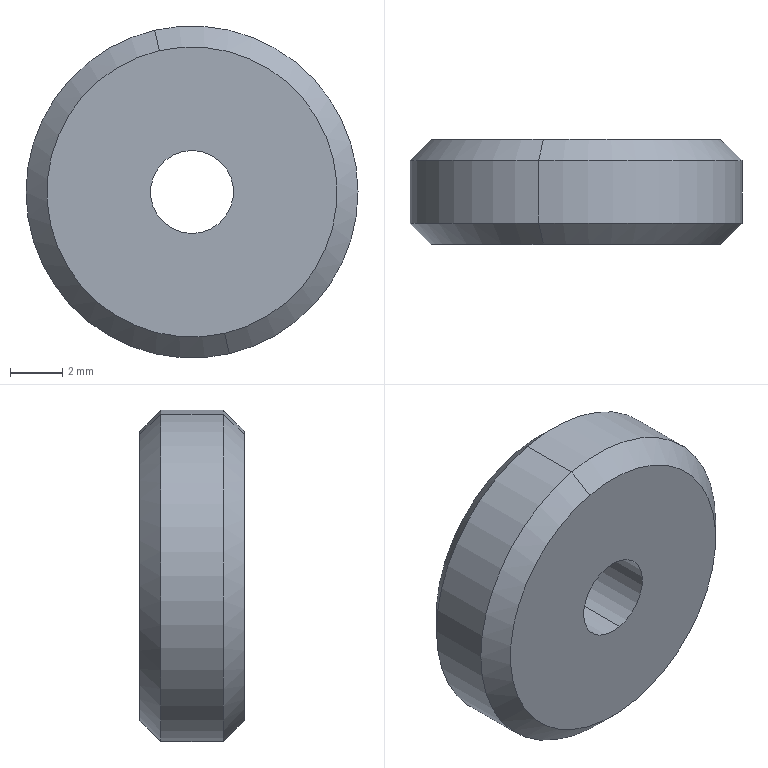Part | STEP file | 4-20.sldasm-Part-188 | 1 solid | 10 faces | box 12.7 x 4 x 12.7 mm | volume 450.576 mm3 | cone 4 | cylinder 4 | plane 2 | commonest cylinder face diameters 3.175 x2 12.7 x2
STEP:
#1=CARTESIAN_POINT('',(-144.626,-599.425,-33.06));
#2=VERTEX_POINT('',#1);
#3=CARTESIAN_POINT('',(-147.122,-599.425,-22.244));
#4=VERTEX_POINT('',#3);
#5=CARTESIAN_POINT('',(-145.874,-599.425,-27.652));
#6=DIRECTION('',(0.,-1.,0.));
#7=DIRECTION('',(-0.225,0.,0.9744));
#8=AXIS2_PLACEMENT_3D('',#5,#6,#7);
#9=CIRCLE('',#8,5.55);
#10=EDGE_CURVE('',#2,#4,#9,.T.);
#11=ORIENTED_EDGE('',*,*,#10,.F.);
#12=CARTESIAN_POINT('',(-144.446,-598.625,-33.84));
#13=VERTEX_POINT('',#12);
#14=CARTESIAN_POINT('',(-144.626,-599.425,-33.06));
#15=DIRECTION('',(0.1591,0.7071,-0.689));
#16=VECTOR('',#15,1000.);
#17=LINE('',#14,#16);
#18=EDGE_CURVE('',#2,#13,#17,.T.);
#19=ORIENTED_EDGE('',*,*,#18,.T.);
#20=CARTESIAN_POINT('',(-147.302,-598.625,-21.465));
#21=VERTEX_POINT('',#20);
#22=CARTESIAN_POINT('',(-145.874,-598.625,-27.652));
#23=DIRECTION('',(0.,1.,0.));
#24=DIRECTION('',(0.225,0.,-0.9744));
#25=AXIS2_PLACEMENT_3D('',#22,#23,#24);
#26=CIRCLE('',#25,6.35);
#27=EDGE_CURVE('',#21,#13,#26,.T.);
#28=ORIENTED_EDGE('',*,*,#27,.F.);
#29=CARTESIAN_POINT('',(-147.122,-599.425,-22.244));
#30=DIRECTION('',(-0.1591,0.7071,0.689));
#31=VECTOR('',#30,1000.);
#32=LINE('',#29,#31);
#33=EDGE_CURVE('',#4,#21,#32,.T.);
#34=ORIENTED_EDGE('',*,*,#33,.F.);
#35=EDGE_LOOP('',(#11,#19,#28,#34));
#36=FACE_OUTER_BOUND('',#35,.T.);
#37=CARTESIAN_POINT('',(-145.874,-599.425,-27.652));
#38=DIRECTION('',(0.,1.,0.));
#39=DIRECTION('',(-0.225,0.,0.9744));
#40=AXIS2_PLACEMENT_3D('',#37,#38,#39);
#41=CONICAL_SURFACE('',#40,5.55,0.7854);
#42=ADVANCED_FACE('',(#36),#41,.T.);
#43=CARTESIAN_POINT('',(-147.122,-595.425,-22.244));
#44=VERTEX_POINT('',#43);
#45=CARTESIAN_POINT('',(-144.626,-595.425,-33.06));
#46=VERTEX_POINT('',#45);
#47=CARTESIAN_POINT('',(-145.874,-595.425,-27.652));
#48=DIRECTION('',(0.,1.,0.));
#49=DIRECTION('',(-0.225,0.,0.9744));
#50=AXIS2_PLACEMENT_3D('',#47,#48,#49);
#51=CIRCLE('',#50,5.55);
#52=EDGE_CURVE('',#44,#46,#51,.T.);
#53=ORIENTED_EDGE('',*,*,#52,.F.);
#54=CARTESIAN_POINT('',(-147.302,-596.225,-21.465));
#55=VERTEX_POINT('',#54);
#56=CARTESIAN_POINT('',(-147.302,-596.225,-21.465));
#57=DIRECTION('',(-0.1591,-0.7071,0.689));
#58=VECTOR('',#57,1000.);
#59=LINE('',#56,#58);
#60=EDGE_CURVE('',#44,#55,#59,.T.);
#61=ORIENTED_EDGE('',*,*,#60,.T.);
#62=CARTESIAN_POINT('',(-144.446,-596.225,-33.84));
#63=VERTEX_POINT('',#62);
#64=CARTESIAN_POINT('',(-145.874,-596.225,-27.652));
#65=DIRECTION('',(0.,-1.,0.));
#66=DIRECTION('',(-0.225,0.,0.9744));
#67=AXIS2_PLACEMENT_3D('',#64,#65,#66);
#68=CIRCLE('',#67,6.35);
#69=EDGE_CURVE('',#63,#55,#68,.T.);
#70=ORIENTED_EDGE('',*,*,#69,.F.);
#71=CARTESIAN_POINT('',(-144.446,-596.225,-33.84));
#72=DIRECTION('',(0.1591,-0.7071,-0.689));
#73=VECTOR('',#72,1000.);
#74=LINE('',#71,#73);
#75=EDGE_CURVE('',#46,#63,#74,.T.);
#76=ORIENTED_EDGE('',*,*,#75,.F.);
#77=EDGE_LOOP('',(#53,#61,#70,#76));
#78=FACE_OUTER_BOUND('',#77,.T.);
#79=CARTESIAN_POINT('',(-145.874,-596.225,-27.652));
#80=DIRECTION('',(0.,-1.,0.));
#81=DIRECTION('',(0.225,0.,-0.9744));
#82=AXIS2_PLACEMENT_3D('',#79,#80,#81);
#83=CONICAL_SURFACE('',#82,6.35,0.7854);
#84=ADVANCED_FACE('',(#78),#83,.T.);
#85=CARTESIAN_POINT('',(-146.231,-599.425,-26.105));
#86=VERTEX_POINT('',#85);
#87=CARTESIAN_POINT('',(-145.517,-599.425,-29.199));
#88=VERTEX_POINT('',#87);
#89=CARTESIAN_POINT('',(-145.874,-599.425,-27.652));
#90=DIRECTION('',(0.,-1.,0.));
#91=DIRECTION('',(0.225,0.,-0.9744));
#92=AXIS2_PLACEMENT_3D('',#89,#90,#91);
#93=CIRCLE('',#92,1.587);
#94=EDGE_CURVE('',#86,#88,#93,.T.);
#95=ORIENTED_EDGE('',*,*,#94,.T.);
#96=CARTESIAN_POINT('',(-145.517,-595.425,-29.199));
#97=VERTEX_POINT('',#96);
#98=CARTESIAN_POINT('',(-145.517,-599.425,-29.199));
#99=DIRECTION('',(0.,1.,0.));
#100=VECTOR('',#99,1000.);
#101=LINE('',#98,#100);
#102=EDGE_CURVE('',#88,#97,#101,.T.);
#103=ORIENTED_EDGE('',*,*,#102,.T.);
#104=CARTESIAN_POINT('',(-146.231,-595.425,-26.105));
#105=VERTEX_POINT('',#104);
#106=CARTESIAN_POINT('',(-145.874,-595.425,-27.652));
#107=DIRECTION('',(0.,-1.,0.));
#108=DIRECTION('',(0.225,0.,-0.9744));
#109=AXIS2_PLACEMENT_3D('',#106,#107,#108);
#110=CIRCLE('',#109,1.587);
#111=EDGE_CURVE('',#105,#97,#110,.T.);
#112=ORIENTED_EDGE('',*,*,#111,.F.);
#113=CARTESIAN_POINT('',(-146.231,-599.425,-26.105));
#114=DIRECTION('',(0.,1.,0.));
#115=VECTOR('',#114,1000.);
#116=LINE('',#113,#115);
#117=EDGE_CURVE('',#86,#105,#116,.T.);
#118=ORIENTED_EDGE('',*,*,#117,.F.);
#119=EDGE_LOOP('',(#95,#103,#112,#118));
#120=FACE_OUTER_BOUND('',#119,.T.);
#121=CARTESIAN_POINT('',(-145.874,-599.425,-27.652));
#122=DIRECTION('',(0.,1.,0.));
#123=DIRECTION('',(-0.225,0.,0.9744));
#124=AXIS2_PLACEMENT_3D('',#121,#122,#123);
#125=CYLINDRICAL_SURFACE('',#124,1.587);
#126=ADVANCED_FACE('',(#120),#125,.F.);
#127=ORIENTED_EDGE('',*,*,#27,.T.);
#128=CARTESIAN_POINT('',(-144.446,-599.425,-33.84));
#129=DIRECTION('',(0.,1.,0.));
#130=VECTOR('',#129,1000.);
#131=LINE('',#128,#130);
#132=EDGE_CURVE('',#13,#63,#131,.T.);
#133=ORIENTED_EDGE('',*,*,#132,.T.);
#134=ORIENTED_EDGE('',*,*,#69,.T.);
#135=CARTESIAN_POINT('',(-147.302,-599.425,-21.465));
#136=DIRECTION('',(0.,1.,0.));
#137=VECTOR('',#136,1000.);
#138=LINE('',#135,#137);
#139=EDGE_CURVE('',#21,#55,#138,.T.);
#140=ORIENTED_EDGE('',*,*,#139,.F.);
#141=EDGE_LOOP('',(#127,#133,#134,#140));
#142=FACE_OUTER_BOUND('',#141,.T.);
#143=CARTESIAN_POINT('',(-145.874,-599.425,-27.652));
#144=DIRECTION('',(0.,1.,0.));
#145=DIRECTION('',(-0.225,0.,0.9744));
#146=AXIS2_PLACEMENT_3D('',#143,#144,#145);
#147=CYLINDRICAL_SURFACE('',#146,6.35);
#148=ADVANCED_FACE('',(#142),#147,.T.);
#149=ORIENTED_EDGE('',*,*,#132,.F.);
#150=CARTESIAN_POINT('',(-145.874,-598.625,-27.652));
#151=DIRECTION('',(0.,1.,0.));
#152=DIRECTION('',(0.225,0.,-0.9744));
#153=AXIS2_PLACEMENT_3D('',#150,#151,#152);
#154=CIRCLE('',#153,6.35);
#155=EDGE_CURVE('',#13,#21,#154,.T.);
#156=ORIENTED_EDGE('',*,*,#155,.T.);
#157=ORIENTED_EDGE('',*,*,#139,.T.);
#158=CARTESIAN_POINT('',(-145.874,-596.225,-27.652));
#159=DIRECTION('',(0.,-1.,0.));
#160=DIRECTION('',(-0.225,0.,0.9744));
#161=AXIS2_PLACEMENT_3D('',#158,#159,#160);
#162=CIRCLE('',#161,6.35);
#163=EDGE_CURVE('',#55,#63,#162,.T.);
#164=ORIENTED_EDGE('',*,*,#163,.T.);
#165=EDGE_LOOP('',(#149,#156,#157,#164));
#166=FACE_OUTER_BOUND('',#165,.T.);
#167=CARTESIAN_POINT('',(-145.874,-599.425,-27.652));
#168=DIRECTION('',(0.,1.,0.));
#169=DIRECTION('',(-0.225,0.,0.9744));
#170=AXIS2_PLACEMENT_3D('',#167,#168,#169);
#171=CYLINDRICAL_SURFACE('',#170,6.35);
#172=ADVANCED_FACE('',(#166),#171,.T.);
#173=CARTESIAN_POINT('',(-145.874,-595.425,-27.652));
#174=DIRECTION('',(0.,1.,0.));
#175=DIRECTION('',(-0.225,0.,0.9744));
#176=AXIS2_PLACEMENT_3D('',#173,#174,#175);
#177=CIRCLE('',#176,5.55);
#178=EDGE_CURVE('',#46,#44,#177,.T.);
#179=ORIENTED_EDGE('',*,*,#178,.T.);
#180=ORIENTED_EDGE('',*,*,#52,.T.);
#181=EDGE_LOOP('',(#179,#180));
#182=FACE_OUTER_BOUND('',#181,.T.);
#183=ORIENTED_EDGE('',*,*,#111,.T.);
#184=CARTESIAN_POINT('',(-145.874,-595.425,-27.652));
#185=DIRECTION('',(0.,-1.,0.));
#186=DIRECTION('',(0.225,0.,-0.9744));
#187=AXIS2_PLACEMENT_3D('',#184,#185,#186);
#188=CIRCLE('',#187,1.587);
#189=EDGE_CURVE('',#97,#105,#188,.T.);
#190=ORIENTED_EDGE('',*,*,#189,.T.);
#191=EDGE_LOOP('',(#183,#190));
#192=FACE_BOUND('',#191,.T.);
#193=CARTESIAN_POINT('',(-145.874,-595.425,-27.652));
#194=DIRECTION('',(0.,1.,0.));
#195=DIRECTION('',(-0.225,0.,0.9744));
#196=AXIS2_PLACEMENT_3D('',#193,#194,#195);
#197=PLANE('',#196);
#198=ADVANCED_FACE('',(#182,#192),#197,.T.);
#199=CARTESIAN_POINT('',(-145.874,-599.425,-27.652));
#200=DIRECTION('',(0.,-1.,0.));
#201=DIRECTION('',(-0.225,0.,0.9744));
#202=AXIS2_PLACEMENT_3D('',#199,#200,#201);
#203=CIRCLE('',#202,5.55);
#204=EDGE_CURVE('',#4,#2,#203,.T.);
#205=ORIENTED_EDGE('',*,*,#204,.T.);
#206=ORIENTED_EDGE('',*,*,#10,.T.);
#207=EDGE_LOOP('',(#205,#206));
#208=FACE_OUTER_BOUND('',#207,.T.);
#209=ORIENTED_EDGE('',*,*,#94,.F.);
#210=CARTESIAN_POINT('',(-145.874,-599.425,-27.652));
#211=DIRECTION('',(0.,-1.,0.));
#212=DIRECTION('',(0.225,0.,-0.9744));
#213=AXIS2_PLACEMENT_3D('',#210,#211,#212);
#214=CIRCLE('',#213,1.587);
#215=EDGE_CURVE('',#88,#86,#214,.T.);
#216=ORIENTED_EDGE('',*,*,#215,.F.);
#217=EDGE_LOOP('',(#209,#216));
#218=FACE_BOUND('',#217,.T.);
#219=CARTESIAN_POINT('',(-145.874,-599.425,-27.652));
#220=DIRECTION('',(0.,1.,0.));
#221=DIRECTION('',(-0.225,0.,0.9744));
#222=AXIS2_PLACEMENT_3D('',#219,#220,#221);
#223=PLANE('',#222);
#224=ADVANCED_FACE('',(#208,#218),#223,.F.);
#225=ORIENTED_EDGE('',*,*,#102,.F.);
#226=ORIENTED_EDGE('',*,*,#215,.T.);
#227=ORIENTED_EDGE('',*,*,#117,.T.);
#228=ORIENTED_EDGE('',*,*,#189,.F.);
#229=EDGE_LOOP('',(#225,#226,#227,#228));
#230=FACE_OUTER_BOUND('',#229,.T.);
#231=CARTESIAN_POINT('',(-145.874,-599.425,-27.652));
#232=DIRECTION('',(0.,1.,0.));
#233=DIRECTION('',(-0.225,0.,0.9744));
#234=AXIS2_PLACEMENT_3D('',#231,#232,#233);
#235=CYLINDRICAL_SURFACE('',#234,1.587);
#236=ADVANCED_FACE('',(#230),#235,.F.);
#237=ORIENTED_EDGE('',*,*,#60,.F.);
#238=ORIENTED_EDGE('',*,*,#178,.F.);
#239=ORIENTED_EDGE('',*,*,#75,.T.);
#240=ORIENTED_EDGE('',*,*,#163,.F.);
#241=EDGE_LOOP('',(#237,#238,#239,#240));
#242=FACE_OUTER_BOUND('',#241,.T.);
#243=CARTESIAN_POINT('',(-145.874,-596.225,-27.652));
#244=DIRECTION('',(0.,-1.,0.));
#245=DIRECTION('',(0.225,0.,-0.9744));
#246=AXIS2_PLACEMENT_3D('',#243,#244,#245);
#247=CONICAL_SURFACE('',#246,6.35,0.7854);
#248=ADVANCED_FACE('',(#242),#247,.T.);
#249=ORIENTED_EDGE('',*,*,#18,.F.);
#250=ORIENTED_EDGE('',*,*,#204,.F.);
#251=ORIENTED_EDGE('',*,*,#33,.T.);
#252=ORIENTED_EDGE('',*,*,#155,.F.);
#253=EDGE_LOOP('',(#249,#250,#251,#252));
#254=FACE_OUTER_BOUND('',#253,.T.);
#255=CARTESIAN_POINT('',(-145.874,-599.425,-27.652));
#256=DIRECTION('',(0.,1.,0.));
#257=DIRECTION('',(-0.225,0.,0.9744));
#258=AXIS2_PLACEMENT_3D('',#255,#256,#257);
#259=CONICAL_SURFACE('',#258,5.55,0.7854);
#260=ADVANCED_FACE('',(#254),#259,.T.);
#261=CLOSED_SHELL('',(#42,#84,#126,#148,#172,#198,#224,#236,#248,#260));
#262=MANIFOLD_SOLID_BREP('',#261);
#263=CARTESIAN_POINT('',(0.,0.,0.));
#264=DIRECTION('',(0.,0.,1.));
#265=DIRECTION('',(1.,0.,0.));
#266=AXIS2_PLACEMENT_3D('',#263,#264,#265);
#267=(LENGTH_UNIT()NAMED_UNIT(*)SI_UNIT(.MILLI.,.METRE.));
#268=UNCERTAINTY_MEASURE_WITH_UNIT(LENGTH_MEASURE(0.00001),#267,'','');
#269=(NAMED_UNIT(*)PLANE_ANGLE_UNIT()SI_UNIT($,.RADIAN.));
#270=(NAMED_UNIT(*)SI_UNIT($,.STERADIAN.)SOLID_ANGLE_UNIT());
#271=(GEOMETRIC_REPRESENTATION_CONTEXT(3)GLOBAL_UNCERTAINTY_ASSIGNED_CONTEXT((#268))GLOBAL_UNIT_ASSIGNED_CONTEXT((#267,#269,#270))REPRESENTATION_CONTEXT('',''));
#272=ADVANCED_BREP_SHAPE_REPRESENTATION('',(#262,#266),#271);